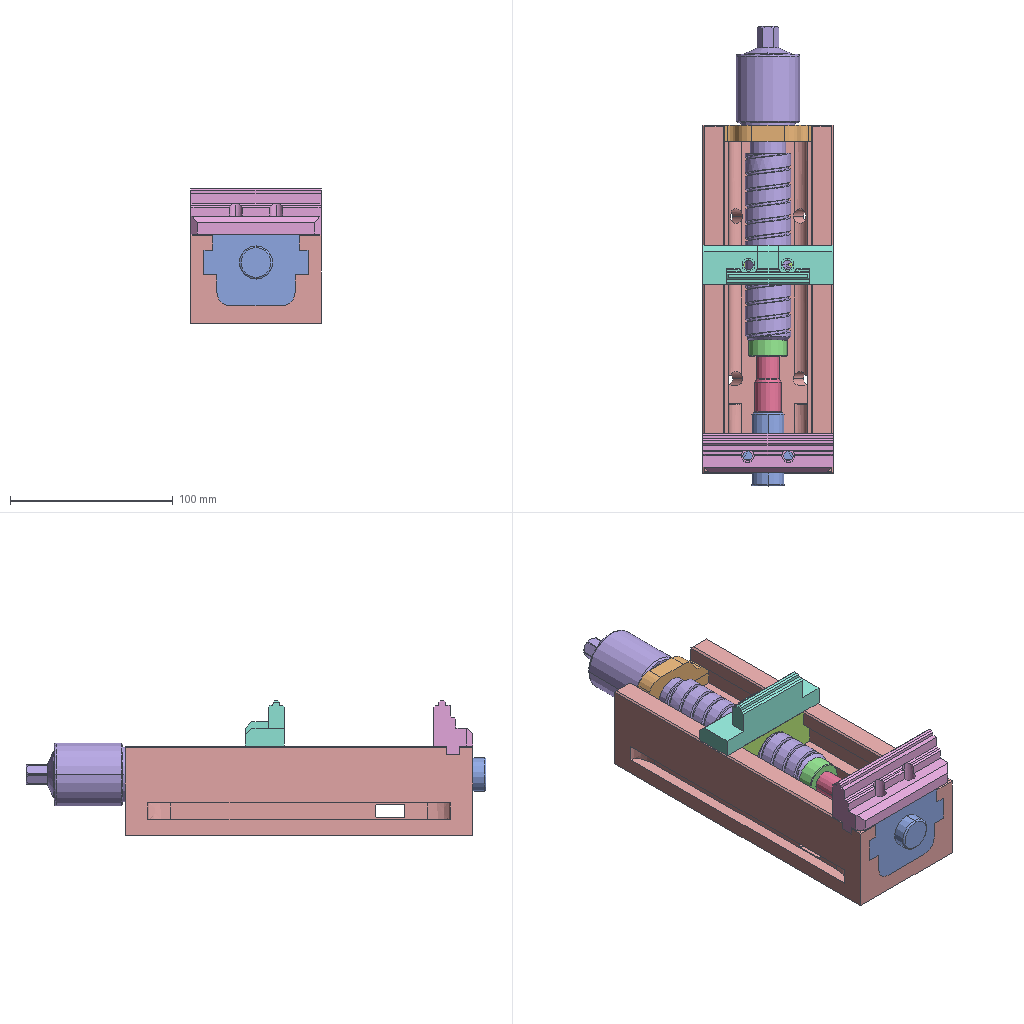Assembly | SolidWorks | 7 different items | 7 placed | box 80 x 283 x 83 mm
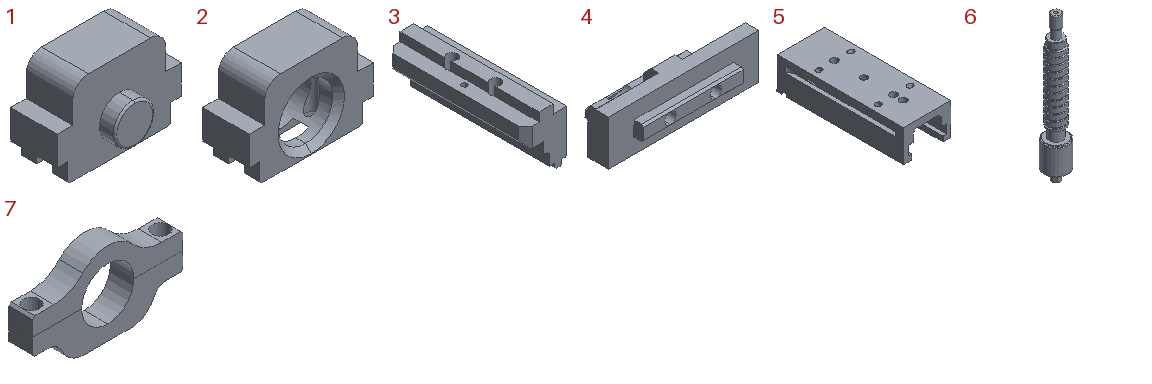Parts list (item | quantity | size | volume | features):
1 | x1 | 64 x 45 x 44 mm | 54258 mm3 | features ICE 5, Chamfer 2, CutThin 1, Draft 1, Extrusion 1, Fillet 1
2 | x1 | 64 x 24 x 44 mm | 38268 mm3 | features ICE 3, Chamfer 2, Extrusion 1
3 | x1 | 24 x 80 x 33 mm | 35961 mm3 | features ICE 4, Chamfer 2, Extrusion 1
4 | x1 | 80 x 33 x 24 mm | 28866 mm3 | features ICE 7, Chamfer 3, Extrusion 1, Fillet 1
5 | x1 | 80 x 214 x 55 mm | 394172 mm3 | features HoleWzd 3, ICE 3, 3DProfileFeature 2, Chamfer 1, Extrusion 1, Fillet 1, MirrorPattern 1
6 | x1 | 39 x 39 x 238 mm | 139894 mm3 | features ICE 3, BaseBody 1, Chamfer 1, Helix 1, MoveCopyBody 1, Split 1, SweepCut 1
7 | x1 | 64 x 10 x 35.214 mm | 11091 mm3 | features ICE 2, Chamfer 1, Extrusion 1, PLine 1
Mates (type | each side: item.copy, entity, surface, feature):
Coincident | 5.1 face plane Boss-Extrude1 | 1.1 face plane Boss-Extrude1 | 2 times
Parallel | 5.1 face plane Boss-Extrude1 | 1.1 face plane Boss-Extrude1
Coincident | 5.1 face plane Cut-Extrude1 | 1.1 face plane Cut-Extrude1
Coincident | 5.1 face plane Boss-Extrude1 | 2.1 face plane Boss-Extrude1 | 2 times
Coincident | 2.1 face plane Boss-Extrude1 | 5.1 face plane Boss-Extrude1
Coincident | 5.1 face plane Boss-Extrude1 | 7.1 face plane Split Line1 | 2 times
Coincident | 5.1 face plane Boss-Extrude1 | 7.1 face plane Boss-Extrude1
Coincident | 1.1 face plane Cut-Extrude1 | 3.1 face plane Boss-Extrude2 | 2 times
Concentric | 2.1 edge | 4.1 edge
Coincident | 2.1 face plane Cut-Extrude1 | 4.1 face plane Boss-Extrude4 | 2 times
Screw | 2.1 edge | 6.1 face cylinder Input1
DistanceDim | 4.1 face plane Boss-Extrude3 | 3.1 face plane Boss-Extrude1
Coincident | 7.1 face plane Split Line1 | 6.1 face plane Boss-Extrude2
Coincident | 7.1 axis | 6.1 axis
PlanarAngleDim | 5.1 face plane Boss-Extrude1 | assembly plane
Coincident | 5.1 face plane Boss-Extrude1 | assembly plane